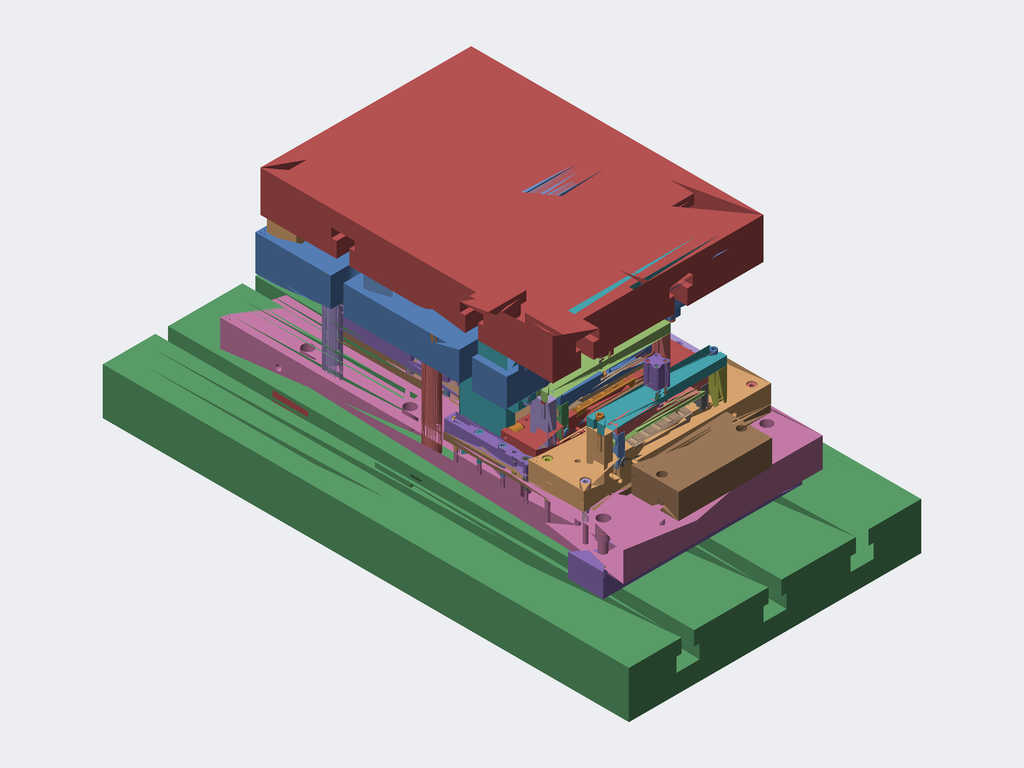Assembly | STEP file | 558 different items | 558 placed
Parts list (item | name | quantity | parent item | size | volume), first 318 of 558 items:
1 | 200 mesh_id1002 | x1 | in 200 mesh_xmt_txt | 10 x 10 x 26 mm | 909.194 mm3
2 | 200 mesh_id1006 | x1 | in 200 mesh_xmt_txt | 10 x 10 x 26 mm | 909.194 mm3
3 | 200 mesh_id1010 | x1 | in 200 mesh_xmt_txt | 10 x 10 x 26 mm | 909.194 mm3
4 | 200 mesh_id1014 | x1 | in 200 mesh_xmt_txt | 10 x 10 x 26 mm | 909.194 mm3
5 | 200 mesh_id1018 | x1 | in 200 mesh_xmt_txt | 10 x 10 x 26 mm | 909.194 mm3
6 | 200 mesh_id1022 | x1 | in 200 mesh_xmt_txt | 10 x 10 x 26 mm | 909.194 mm3
7 | 200 mesh_id1026 | x1 | in 200 mesh_xmt_txt | 10 x 10 x 21 mm | 806.082 mm3
8 | 200 mesh_id102_x | x1 | in 200 mesh_xmt_txt | 6 x 6 x 36.5 mm | 342.508 mm3
9 | 200 mesh_id1030 | x1 | in 200 mesh_xmt_txt | 10 x 10 x 21 mm | 806.082 mm3
10 | 200 mesh_id1034 | x1 | in 200 mesh_xmt_txt | 10 x 10 x 21 mm | 806.082 mm3
11 | 200 mesh_id1038 | x1 | in 200 mesh_xmt_txt | 10 x 10 x 21 mm | 806.082 mm3
12 | 200 mesh_id1042 | x1 | in 200 mesh_xmt_txt | 10 x 10 x 21 mm | 806.082 mm3
13 | 200 mesh_id1046 | x1 | in 200 mesh_xmt_txt | 6 x 6 x 24.2 mm | 255.883 mm3
14 | 200 mesh_id1050 | x1 | in 200 mesh_xmt_txt | 6 x 6 x 24.2 mm | 255.883 mm3
15 | 200 mesh_id1054 | x1 | in 200 mesh_xmt_txt | 6 x 6 x 24.2 mm | 255.883 mm3
16 | 200 mesh_id1058 | x1 | in 200 mesh_xmt_txt | 6 x 6 x 24.2 mm | 255.883 mm3
17 | 200 mesh_id1062 | x1 | in 200 mesh_xmt_txt | 6 x 6 x 24.2 mm | 255.883 mm3
18 | 200 mesh_id1066 | x1 | in 200 mesh_xmt_txt | 6 x 6 x 24.2 mm | 255.883 mm3
19 | 200 mesh_id106_x | x1 | in 200 mesh_xmt_txt | 6 x 6 x 36.5 mm | 342.508 mm3
20 | 200 mesh_id1070 | x1 | in 200 mesh_xmt_txt | 6 x 6 x 24.2 mm | 255.883 mm3
21 | 200 mesh_id1074 | x1 | in 200 mesh_xmt_txt | 6 x 6 x 24.2 mm | 255.883 mm3
22 | 200 mesh_id1078 | x1 | in 200 mesh_xmt_txt | 6 x 6 x 24.2 mm | 255.883 mm3
23 | 200 mesh_id1082 | x1 | in 200 mesh_xmt_txt | 6 x 6 x 24.2 mm | 255.883 mm3
24 | 200 mesh_id1086 | x1 | in 200 mesh_xmt_txt | 6 x 6 x 24.2 mm | 255.883 mm3
25 | 200 mesh_id1090 | x1 | in 200 mesh_xmt_txt | 6 x 6 x 24.2 mm | 255.883 mm3
26 | 200 mesh_id1094 | x1 | in 200 mesh_xmt_txt | 6 x 6 x 24.2 mm | 255.883 mm3
27 | 200 mesh_id1098 | x1 | in 200 mesh_xmt_txt | 6 x 6 x 24.2 mm | 255.883 mm3
28 | 200 mesh_id10_xmt | x1 | in 200 mesh_xmt_txt | 60 x 14 x 9.8 mm | 6516 mm3
29 | 200 mesh_id1102 | x1 | in 200 mesh_xmt_txt | 6 x 6 x 24.2 mm | 255.883 mm3
30 | 200 mesh_id1106 | x1 | in 200 mesh_xmt_txt | 6 x 6 x 24.2 mm | 255.883 mm3
31 | 200 mesh_id110_x | x1 | in 200 mesh_xmt_txt | 6 x 6 x 36.5 mm | 342.508 mm3
32 | 200 mesh_id1110 | x1 | in 200 mesh_xmt_txt | 6 x 6 x 24.2 mm | 255.883 mm3
33 | 200 mesh_id1114 | x1 | in 200 mesh_xmt_txt | 6 x 6 x 24.2 mm | 255.883 mm3
34 | 200 mesh_id1118 | x1 | in 200 mesh_xmt_txt | 6 x 6 x 33.5 mm | 321.621 mm3
35 | 200 mesh_id1122 | x1 | in 200 mesh_xmt_txt | 6 x 6 x 33.5 mm | 321.621 mm3
36 | 200 mesh_id1126 | x1 | in 200 mesh_xmt_txt | 6 x 6 x 33.5 mm | 321.621 mm3
37 | 200 mesh_id1130 | x1 | in 200 mesh_xmt_txt | 6 x 6 x 33.5 mm | 321.621 mm3
38 | 200 mesh_id1134 | x1 | in 200 mesh_xmt_txt | 6 x 6 x 33.5 mm | 321.621 mm3
39 | 200 mesh_id1138 | x1 | in 200 mesh_xmt_txt | 6 x 6 x 33.5 mm | 321.621 mm3
40 | 200 mesh_id1142 | x1 | in 200 mesh_xmt_txt | 6 x 6 x 33.5 mm | 321.621 mm3
41 | 200 mesh_id1146 | x1 | in 200 mesh_xmt_txt | 6 x 6 x 33.5 mm | 321.621 mm3
42 | 200 mesh_id114_x | x1 | in 200 mesh_xmt_txt | 6 x 6 x 36.5 mm | 342.508 mm3
43 | 200 mesh_id1150 | x1 | in 200 mesh_xmt_txt | 6 x 6 x 33.5 mm | 321.621 mm3
44 | 200 mesh_id1154 | x1 | in 200 mesh_xmt_txt | 6 x 6 x 33.5 mm | 321.621 mm3
45 | 200 mesh_id1158 | x1 | in 200 mesh_xmt_txt | 6 x 6 x 33.5 mm | 321.621 mm3
46 | 200 mesh_id1162 | x1 | in 200 mesh_xmt_txt | 6 x 6 x 33.5 mm | 321.621 mm3
47 | 200 mesh_id1166 | x1 | in 200 mesh_xmt_txt | 6 x 6 x 33.5 mm | 321.621 mm3
48 | 200 mesh_id1170 | x1 | in 200 mesh_xmt_txt | 6 x 6 x 33.5 mm | 321.621 mm3
49 | 200 mesh_id1174 | x1 | in 200 mesh_xmt_txt | 6 x 6 x 33.5 mm | 321.621 mm3
50 | 200 mesh_id1178 | x1 | in 200 mesh_xmt_txt | 6 x 6 x 33.5 mm | 321.621 mm3
51 | 200 mesh_id1182 | x1 | in 200 mesh_xmt_txt | 6 x 6 x 31.5 mm | 307.483 mm3
52 | 200 mesh_id1186 | x1 | in 200 mesh_xmt_txt | 6 x 6 x 31.5 mm | 307.483 mm3
53 | 200 mesh_id118_x | x1 | in 200 mesh_xmt_txt | 6 x 6 x 36.5 mm | 342.508 mm3
54 | 200 mesh_id1190 | x1 | in 200 mesh_xmt_txt | 6 x 6 x 31.5 mm | 307.483 mm3
55 | 200 mesh_id1194 | x1 | in 200 mesh_xmt_txt | 6 x 6 x 31.5 mm | 307.483 mm3
56 | 200 mesh_id1198 | x1 | in 200 mesh_xmt_txt | 6 x 6 x 31.5 mm | 307.483 mm3
57 | 200 mesh_id1202 | x1 | in 200 mesh_xmt_txt | 6 x 6 x 31.5 mm | 307.483 mm3
58 | 200 mesh_id1206 | x1 | in 200 mesh_xmt_txt | 6 x 6 x 31.5 mm | 307.483 mm3
59 | 200 mesh_id1210 | x1 | in 200 mesh_xmt_txt | 6 x 6 x 31.5 mm | 307.483 mm3
60 | 200 mesh_id1214 | x1 | in 200 mesh_xmt_txt | 6 x 6 x 31.5 mm | 307.483 mm3
61 | 200 mesh_id1218 | x1 | in 200 mesh_xmt_txt | 6 x 6 x 31.5 mm | 307.483 mm3
62 | 200 mesh_id1222 | x1 | in 200 mesh_xmt_txt | 6 x 6 x 31.5 mm | 307.483 mm3
63 | 200 mesh_id1226 | x1 | in 200 mesh_xmt_txt | 6 x 6 x 31.5 mm | 307.483 mm3
64 | 200 mesh_id122_x | x1 | in 200 mesh_xmt_txt | 8 x 8 x 55 mm | 2726 mm3
65 | 200 mesh_id1230 | x1 | in 200 mesh_xmt_txt | 6 x 6 x 31.5 mm | 307.483 mm3
66 | 200 mesh_id1234 | x1 | in 200 mesh_xmt_txt | 6 x 6 x 31.5 mm | 307.483 mm3
67 | 200 mesh_id1238 | x1 | in 200 mesh_xmt_txt | 10 x 10 x 21 mm | 805.584 mm3
68 | 200 mesh_id1242 | x1 | in 200 mesh_xmt_txt | 8.5 x 8.5 x 45 mm | 1026 mm3
69 | 200 mesh_id1246 | x1 | in 200 mesh_xmt_txt | 8.5 x 8.5 x 45 mm | 1026 mm3
70 | 200 mesh_id1250 | x1 | in 200 mesh_xmt_txt | 39.94 x 2.4 x 27.2 mm | 2495 mm3
71 | 200 mesh_id1254 | x1 | in 200 mesh_xmt_txt | 39.94 x 2.4 x 27.2 mm | 2495 mm3
72 | 200 mesh_id1258 | x1 | in 200 mesh_xmt_txt | 39.94 x 2.4 x 27.2 mm | 2495 mm3
73 | 200 mesh_id1262 | x1 | in 200 mesh_xmt_txt | 39.94 x 2.4 x 27.2 mm | 2495 mm3
74 | 200 mesh_id1266 | x1 | in 200 mesh_xmt_txt | 39.94 x 2.4 x 27.2 mm | 2495 mm3
75 | 200 mesh_id126_x | x1 | in 200 mesh_xmt_txt | 10 x 10 x 21 mm | 805.776 mm3
76 | 200 mesh_id1270 | x1 | in 200 mesh_xmt_txt | 39.94 x 2.4 x 27.2 mm | 2495 mm3
77 | 200 mesh_id1274 | x1 | in 200 mesh_xmt_txt | 39.94 x 2.4 x 27.2 mm | 2495 mm3
78 | 200 mesh_id1278 | x1 | in 200 mesh_xmt_txt | 39.94 x 2.4 x 27.2 mm | 2495 mm3
79 | 200 mesh_id1282 | x1 | in 200 mesh_xmt_txt | 39.94 x 2.4 x 27.2 mm | 2495 mm3
80 | 200 mesh_id1286 | x1 | in 200 mesh_xmt_txt | 39.94 x 2.4 x 27.2 mm | 2495 mm3
81 | 200 mesh_id1290 | x1 | in 200 mesh_xmt_txt | 39.94 x 2.4 x 27.2 mm | 2495 mm3
82 | 200 mesh_id1294 | x1 | in 200 mesh_xmt_txt | 39.94 x 2.4 x 27.2 mm | 2495 mm3
83 | 200 mesh_id1298 | x1 | in 200 mesh_xmt_txt | 39.94 x 2.4 x 27.2 mm | 2495 mm3
84 | 200 mesh_id1302 | x1 | in 200 mesh_xmt_txt | 39.94 x 2.4 x 27.2 mm | 2495 mm3
85 | 200 mesh_id1306 | x1 | in 200 mesh_xmt_txt | 39.94 x 2.4 x 27.2 mm | 2495 mm3
86 | 200 mesh_id130_x | x1 | in 200 mesh_xmt_txt | 8.5 x 8.5 x 20 mm | 535.142 mm3
87 | 200 mesh_id1310 | x1 | in 200 mesh_xmt_txt | 39.94 x 2.4 x 27.2 mm | 2495 mm3
88 | 200 mesh_id1314 | x1 | in 200 mesh_xmt_txt | 39.94 x 2.4 x 27.2 mm | 2495 mm3
89 | 200 mesh_id1318 | x1 | in 200 mesh_xmt_txt | 39.94 x 2.4 x 27.2 mm | 2495 mm3
90 | 200 mesh_id1322 | x1 | in 200 mesh_xmt_txt | 22 x 22 x 5 mm | 1608 mm3
91 | 200 mesh_id1326 | x1 | in 200 mesh_xmt_txt | 12 x 12 x 32.3 mm | 2576 mm3
92 | 200 mesh_id1330 | x1 | in 200 mesh_xmt_txt | 12 x 12 x 32.3 mm | 2576 mm3
93 | 200 mesh_id1334 | x1 | in 200 mesh_xmt_txt | 22 x 22 x 5 mm | 1608 mm3
94 | 200 mesh_id1338 | x1 | in 200 mesh_xmt_txt | 12 x 12 x 32.3 mm | 2576 mm3
95 | 200 mesh_id1342 | x1 | in 200 mesh_xmt_txt | 22 x 22 x 5 mm | 1608 mm3
96 | 200 mesh_id1346 | x1 | in 200 mesh_xmt_txt | 12 x 12 x 32.3 mm | 2576 mm3
97 | 200 mesh_id134_x | x1 | in 200 mesh_xmt_txt | 10 x 10 x 51 mm | 1654 mm3
98 | 200 mesh_id1350 | x1 | in 200 mesh_xmt_txt | 22 x 22 x 5 mm | 1608 mm3
99 | 200 mesh_id1354 | x1 | in 200 mesh_xmt_txt | 22 x 22 x 5 mm | 1608 mm3
100 | 200 mesh_id1358 | x1 | in 200 mesh_xmt_txt | 12 x 12 x 32.3 mm | 2576 mm3
101 | 200 mesh_id1362 | x1 | in 200 mesh_xmt_txt | 22 x 22 x 5 mm | 1608 mm3
102 | 200 mesh_id1366 | x1 | in 200 mesh_xmt_txt | 12 x 12 x 32.3 mm | 2576 mm3
103 | 200 mesh_id1370 | x1 | in 200 mesh_xmt_txt | 8 x 8 x 10 mm | 413.018 mm3
104 | 200 mesh_id1374 | x1 | in 200 mesh_xmt_txt | 8 x 8 x 10 mm | 413.018 mm3
105 | 200 mesh_id1378 | x1 | in 200 mesh_xmt_txt | 8 x 8 x 10 mm | 413.018 mm3
106 | 200 mesh_id1382 | x1 | in 200 mesh_xmt_txt | 8 x 8 x 10 mm | 413.018 mm3
107 | 200 mesh_id1386 | x1 | in 200 mesh_xmt_txt | 8 x 8 x 10 mm | 413.018 mm3
108 | 200 mesh_id138_x | x1 | in 200 mesh_xmt_txt | 18 x 18 x 30 mm | 2880 mm3
109 | 200 mesh_id1390 | x1 | in 200 mesh_xmt_txt | 8 x 8 x 10 mm | 413.018 mm3
110 | 200 mesh_id1394 | x1 | in 200 mesh_xmt_txt | 8 x 8 x 10 mm | 413.018 mm3
111 | 200 mesh_id1398 | x1 | in 200 mesh_xmt_txt | 8 x 8 x 10 mm | 413.018 mm3
112 | 200 mesh_id1402 | x1 | in 200 mesh_xmt_txt | 8 x 8 x 10 mm | 413.018 mm3
113 | 200 mesh_id1406 | x1 | in 200 mesh_xmt_txt | 8 x 8 x 10 mm | 413.018 mm3
114 | 200 mesh_id1410 | x1 | in 200 mesh_xmt_txt | 8 x 8 x 10 mm | 413.018 mm3
115 | 200 mesh_id1414 | x1 | in 200 mesh_xmt_txt | 8 x 8 x 10 mm | 413.018 mm3
116 | 200 mesh_id1418 | x1 | in 200 mesh_xmt_txt | 8 x 8 x 10 mm | 413.018 mm3
117 | 200 mesh_id1422 | x1 | in 200 mesh_xmt_txt | 8 x 8 x 10 mm | 413.018 mm3
118 | 200 mesh_id1426 | x1 | in 200 mesh_xmt_txt | 8 x 8 x 10 mm | 413.018 mm3
119 | 200 mesh_id142_x | x1 | in 200 mesh_xmt_txt | 18 x 18 x 30 mm | 2880 mm3
120 | 200 mesh_id1430 | x1 | in 200 mesh_xmt_txt | 8 x 8 x 10 mm | 413.018 mm3
121 | 200 mesh_id1434 | x1 | in 200 mesh_xmt_txt | 8 x 8 x 10 mm | 413.018 mm3
122 | 200 mesh_id1438 | x1 | in 200 mesh_xmt_txt | 8 x 8 x 10 mm | 413.018 mm3
123 | 200 mesh_id1442 | x1 | in 200 mesh_xmt_txt | 8 x 8 x 10 mm | 413.018 mm3
124 | 200 mesh_id1446 | x1 | in 200 mesh_xmt_txt | 8 x 8 x 10 mm | 413.018 mm3
125 | 200 mesh_id1450 | x1 | in 200 mesh_xmt_txt | 8 x 8 x 10 mm | 413.018 mm3
126 | 200 mesh_id1454 | x1 | in 200 mesh_xmt_txt | 8 x 8 x 10 mm | 413.018 mm3
127 | 200 mesh_id1458 | x1 | in 200 mesh_xmt_txt | 8 x 8 x 10 mm | 413.018 mm3
128 | 200 mesh_id1462 | x1 | in 200 mesh_xmt_txt | 8 x 8 x 10 mm | 413.018 mm3
129 | 200 mesh_id1466 | x1 | in 200 mesh_xmt_txt | 8 x 8 x 10 mm | 413.018 mm3
130 | 200 mesh_id146_x | x1 | in 200 mesh_xmt_txt | 18 x 18 x 30 mm | 2880 mm3
131 | 200 mesh_id1470 | x1 | in 200 mesh_xmt_txt | 8 x 8 x 10 mm | 413.018 mm3
132 | 200 mesh_id1474 | x1 | in 200 mesh_xmt_txt | 8 x 8 x 10 mm | 413.018 mm3
133 | 200 mesh_id1478 | x1 | in 200 mesh_xmt_txt | 8 x 8 x 10 mm | 413.018 mm3
134 | 200 mesh_id1482 | x1 | in 200 mesh_xmt_txt | 8 x 8 x 10 mm | 413.018 mm3
135 | 200 mesh_id1486 | x1 | in 200 mesh_xmt_txt | 8 x 8 x 10 mm | 413.018 mm3
136 | 200 mesh_id1490 | x1 | in 200 mesh_xmt_txt | 8 x 8 x 10 mm | 413.018 mm3
137 | 200 mesh_id1494 | x1 | in 200 mesh_xmt_txt | 8 x 8 x 10 mm | 413.018 mm3
138 | 200 mesh_id1498 | x1 | in 200 mesh_xmt_txt | 8 x 8 x 10 mm | 413.018 mm3
139 | 200 mesh_id14_xmt | x1 | in 200 mesh_xmt_txt | 34.97 x 6 x 32.7 mm | 4654 mm3
140 | 200 mesh_id1502 | x1 | in 200 mesh_xmt_txt | 8 x 8 x 10 mm | 413.018 mm3
141 | 200 mesh_id1506 | x1 | in 200 mesh_xmt_txt | 8 x 8 x 10 mm | 413.018 mm3
142 | 200 mesh_id150_x | x1 | in 200 mesh_xmt_txt | 18 x 18 x 30 mm | 2880 mm3
143 | 200 mesh_id1510 | x1 | in 200 mesh_xmt_txt | 8 x 8 x 10 mm | 413.018 mm3
144 | 200 mesh_id1514 | x1 | in 200 mesh_xmt_txt | 8 x 8 x 10 mm | 413.018 mm3
145 | 200 mesh_id1518 | x1 | in 200 mesh_xmt_txt | 8 x 8 x 10 mm | 413.018 mm3
146 | 200 mesh_id1522 | x1 | in 200 mesh_xmt_txt | 8 x 8 x 10 mm | 413.018 mm3
147 | 200 mesh_id1526 | x1 | in 200 mesh_xmt_txt | 8 x 8 x 10 mm | 413.018 mm3
148 | 200 mesh_id1530 | x1 | in 200 mesh_xmt_txt | 8 x 8 x 10 mm | 413.018 mm3
149 | 200 mesh_id1534 | x1 | in 200 mesh_xmt_txt | 8 x 8 x 10 mm | 413.018 mm3
150 | 200 mesh_id1538 | x1 | in 200 mesh_xmt_txt | 8 x 8 x 10 mm | 413.018 mm3
151 | 200 mesh_id1542 | x1 | in 200 mesh_xmt_txt | 8 x 8 x 10 mm | 413.018 mm3
152 | 200 mesh_id1546 | x1 | in 200 mesh_xmt_txt | 8 x 8 x 10 mm | 413.018 mm3
153 | 200 mesh_id154_x | x1 | in 200 mesh_xmt_txt | 18 x 18 x 30 mm | 2880 mm3
154 | 200 mesh_id1550 | x1 | in 200 mesh_xmt_txt | 8 x 8 x 10 mm | 413.018 mm3
155 | 200 mesh_id1554 | x1 | in 200 mesh_xmt_txt | 8 x 8 x 10 mm | 413.018 mm3
156 | 200 mesh_id1558 | x1 | in 200 mesh_xmt_txt | 24.97 x 5.97 x 53 mm | 7855 mm3
157 | 200 mesh_id1562 | x1 | in 200 mesh_xmt_txt | 6 x 6 x 40 mm | 281.63 mm3
158 | 200 mesh_id1566 | x1 | in 200 mesh_xmt_txt | 6 x 6 x 40 mm | 281.63 mm3
159 | 200 mesh_id1570 | x1 | in 200 mesh_xmt_txt | 6 x 6 x 40 mm | 281.63 mm3
160 | 200 mesh_id1574 | x1 | in 200 mesh_xmt_txt | 6 x 6 x 40 mm | 281.63 mm3
161 | 200 mesh_id1578 | x1 | in 200 mesh_xmt_txt | 6 x 6 x 40 mm | 281.63 mm3
162 | 200 mesh_id1582 | x1 | in 200 mesh_xmt_txt | 6 x 6 x 40 mm | 281.63 mm3
163 | 200 mesh_id1586 | x1 | in 200 mesh_xmt_txt | 6 x 6 x 40 mm | 281.63 mm3
164 | 200 mesh_id158_x | x1 | in 200 mesh_xmt_txt | 18 x 18 x 30 mm | 2880 mm3
165 | 200 mesh_id1590 | x1 | in 200 mesh_xmt_txt | 6 x 6 x 40 mm | 281.63 mm3
166 | 200 mesh_id1594 | x1 | in 200 mesh_xmt_txt | 6 x 6 x 40 mm | 281.63 mm3
167 | 200 mesh_id1598 | x1 | in 200 mesh_xmt_txt | 6 x 6 x 40 mm | 281.63 mm3
168 | 200 mesh_id1602 | x1 | in 200 mesh_xmt_txt | 6 x 6 x 40 mm | 281.63 mm3
169 | 200 mesh_id1606 | x1 | in 200 mesh_xmt_txt | 6 x 6 x 40 mm | 281.63 mm3
170 | 200 mesh_id1610 | x1 | in 200 mesh_xmt_txt | 6 x 6 x 40 mm | 281.63 mm3
171 | 200 mesh_id1614 | x1 | in 200 mesh_xmt_txt | 6 x 6 x 40 mm | 281.63 mm3
172 | 200 mesh_id1618 | x1 | in 200 mesh_xmt_txt | - | 70.891 mm3
173 | 200 mesh_id1622 | x1 | in 200 mesh_xmt_txt | - | 70.891 mm3
174 | 200 mesh_id1626 | x1 | in 200 mesh_xmt_txt | - | 70.891 mm3
175 | 200 mesh_id162_x | x1 | in 200 mesh_xmt_txt | 25 x 25 x 5 mm | 2168 mm3
176 | 200 mesh_id1630 | x1 | in 200 mesh_xmt_txt | - | 70.891 mm3
177 | 200 mesh_id1634 | x1 | in 200 mesh_xmt_txt | - | 70.891 mm3
178 | 200 mesh_id1638 | x1 | in 200 mesh_xmt_txt | - | 70.891 mm3
179 | 200 mesh_id1642 | x1 | in 200 mesh_xmt_txt | - | 70.891 mm3
180 | 200 mesh_id1646 | x1 | in 200 mesh_xmt_txt | - | 70.891 mm3
181 | 200 mesh_id1650 | x1 | in 200 mesh_xmt_txt | - | 70.891 mm3
182 | 200 mesh_id1654 | x1 | in 200 mesh_xmt_txt | - | 70.891 mm3
183 | 200 mesh_id1658 | x1 | in 200 mesh_xmt_txt | - | 70.891 mm3
184 | 200 mesh_id1662 | x1 | in 200 mesh_xmt_txt | - | 70.891 mm3
185 | 200 mesh_id1666 | x1 | in 200 mesh_xmt_txt | - | 70.891 mm3
186 | 200 mesh_id166_x | x1 | in 200 mesh_xmt_txt | 16 x 16 x 25 mm | 3601 mm3
187 | 200 mesh_id1670 | x1 | in 200 mesh_xmt_txt | - | 70.891 mm3
188 | 200 mesh_id1674 | x1 | in 200 mesh_xmt_txt | - | 70.891 mm3
189 | 200 mesh_id1678 | x1 | in 200 mesh_xmt_txt | - | 70.891 mm3
190 | 200 mesh_id1682 | x1 | in 200 mesh_xmt_txt | - | 70.891 mm3
191 | 200 mesh_id1686 | x1 | in 200 mesh_xmt_txt | - | 65.446 mm3
192 | 200 mesh_id1690 | x1 | in 200 mesh_xmt_txt | - | 65.446 mm3
193 | 200 mesh_id1694 | x1 | in 200 mesh_xmt_txt | - | 65.446 mm3
194 | 200 mesh_id1698 | x1 | in 200 mesh_xmt_txt | - | 65.446 mm3
195 | 200 mesh_id1702 | x1 | in 200 mesh_xmt_txt | - | 65.446 mm3
196 | 200 mesh_id1706 | x1 | in 200 mesh_xmt_txt | - | 65.446 mm3
197 | 200 mesh_id170_x | x1 | in 200 mesh_xmt_txt | 25 x 25 x 5 mm | 2168 mm3
198 | 200 mesh_id1710 | x1 | in 200 mesh_xmt_txt | - | 65.446 mm3
199 | 200 mesh_id1714 | x1 | in 200 mesh_xmt_txt | - | 65.446 mm3
200 | 200 mesh_id1718 | x1 | in 200 mesh_xmt_txt | - | 65.446 mm3
201 | 200 mesh_id1722 | x1 | in 200 mesh_xmt_txt | - | 65.446 mm3
202 | 200 mesh_id1726 | x1 | in 200 mesh_xmt_txt | - | 65.446 mm3
203 | 200 mesh_id1730 | x1 | in 200 mesh_xmt_txt | - | 65.446 mm3
204 | 200 mesh_id1734 | x1 | in 200 mesh_xmt_txt | - | 65.446 mm3
205 | 200 mesh_id1738 | x1 | in 200 mesh_xmt_txt | - | 65.446 mm3
206 | 200 mesh_id1742 | x1 | in 200 mesh_xmt_txt | - | 65.446 mm3
207 | 200 mesh_id1746 | x1 | in 200 mesh_xmt_txt | - | 65.446 mm3
208 | 200 mesh_id174_x | x1 | in 200 mesh_xmt_txt | 16 x 16 x 25 mm | 3601 mm3
209 | 200 mesh_id1750 | x1 | in 200 mesh_xmt_txt | - | 65.446 mm3
210 | 200 mesh_id1754 | x1 | in 200 mesh_xmt_txt | - | 65.446 mm3
211 | 200 mesh_id1758 | x1 | in 200 mesh_xmt_txt | 25 x 25 x 45 mm | 5947 mm3
212 | 200 mesh_id1762 | x1 | in 200 mesh_xmt_txt | 25 x 25 x 45 mm | 5947 mm3
213 | 200 mesh_id1766 | x1 | in 200 mesh_xmt_txt | 25 x 25 x 45 mm | 5947 mm3
214 | 200 mesh_id1770 | x1 | in 200 mesh_xmt_txt | 25 x 25 x 45 mm | 5947 mm3
215 | 200 mesh_id1774 | x1 | in 200 mesh_xmt_txt | 25 x 25 x 45 mm | 5947 mm3
216 | 200 mesh_id1778 | x1 | in 200 mesh_xmt_txt | 25 x 25 x 45 mm | 5947 mm3
217 | 200 mesh_id1782 | x1 | in 200 mesh_xmt_txt | 25 x 25 x 45 mm | 5947 mm3
218 | 200 mesh_id1786 | x1 | in 200 mesh_xmt_txt | 25 x 25 x 45 mm | 5947 mm3
219 | 200 mesh_id178_x | x1 | in 200 mesh_xmt_txt | 25 x 25 x 5 mm | 2168 mm3
220 | 200 mesh_id1790 | x1 | in 200 mesh_xmt_txt | 28 x 28 x 30 mm | 6929 mm3
221 | 200 mesh_id1794 | x1 | in 200 mesh_xmt_txt | 22 x 21.896 x 30 mm | 3861 mm3
222 | 200 mesh_id1798 | x1 | in 200 mesh_xmt_txt | 23 x 23 x 140 mm | 28914 mm3
223 | 200 mesh_id1802 | x1 | in 200 mesh_xmt_txt | 21.896 x 22 x 30 mm | 3781 mm3
224 | 200 mesh_id1806 | x1 | in 200 mesh_xmt_txt | 28 x 28 x 35 mm | 8107 mm3
225 | 200 mesh_id1810 | x1 | in 200 mesh_xmt_txt | 28 x 28 x 35 mm | 8107 mm3
226 | 200 mesh_id1814 | x1 | in 200 mesh_xmt_txt | 23 x 23 x 140 mm | 28914 mm3
227 | 200 mesh_id1818 | x1 | in 200 mesh_xmt_txt | 21.896 x 22 x 30 mm | 3781 mm3
228 | 200 mesh_id1822 | x1 | in 200 mesh_xmt_txt | 28 x 28 x 30 mm | 6929 mm3
229 | 200 mesh_id1826 | x1 | in 200 mesh_xmt_txt | 22 x 21.896 x 30 mm | 3861 mm3
230 | 200 mesh_id182_x | x1 | in 200 mesh_xmt_txt | 16 x 16 x 25 mm | 3601 mm3
231 | 200 mesh_id1830 | x1 | in 200 mesh_xmt_txt | 28 x 28 x 35 mm | 8107 mm3
232 | 200 mesh_id1834 | x1 | in 200 mesh_xmt_txt | 23 x 23 x 140 mm | 28914 mm3
233 | 200 mesh_id1838 | x1 | in 200 mesh_xmt_txt | 21.896 x 22 x 30 mm | 3781 mm3
234 | 200 mesh_id1842 | x1 | in 200 mesh_xmt_txt | 22 x 21.896 x 30 mm | 3861 mm3
235 | 200 mesh_id1846 | x1 | in 200 mesh_xmt_txt | 28 x 28 x 30 mm | 6929 mm3
236 | 200 mesh_id1850 | x1 | in 200 mesh_xmt_txt | 28 x 28 x 30 mm | 6929 mm3
237 | 200 mesh_id1854 | x1 | in 200 mesh_xmt_txt | 22 x 21.896 x 30 mm | 3861 mm3
238 | 200 mesh_id1858 | x1 | in 200 mesh_xmt_txt | 23 x 23 x 140 mm | 28914 mm3
239 | 200 mesh_id1862 | x1 | in 200 mesh_xmt_txt | 28 x 28 x 35 mm | 8107 mm3
240 | 200 mesh_id1866 | x1 | in 200 mesh_xmt_txt | 21.896 x 22 x 30 mm | 3781 mm3
241 | 200 mesh_id186_x | x1 | in 200 mesh_xmt_txt | 25 x 25 x 5 mm | 2168 mm3
242 | 200 mesh_id1870 | x1 | in 200 mesh_xmt_txt | 75.6 x 4.94 x 20.309 mm | 3191 mm3
243 | 200 mesh_id1874 | x1 | in 200 mesh_xmt_txt | 75.6 x 4.94 x 20.309 mm | 3191 mm3
244 | 200 mesh_id1878 | x1 | in 200 mesh_xmt_txt | 75.6 x 4.94 x 20.309 mm | 3191 mm3
245 | 200 mesh_id1882 | x1 | in 200 mesh_xmt_txt | 75.6 x 4.94 x 20.309 mm | 3191 mm3
246 | 200 mesh_id1886 | x1 | in 200 mesh_xmt_txt | 90 x 4.94 x 26.94 mm | 4137 mm3
247 | 200 mesh_id1890 | x1 | in 200 mesh_xmt_txt | 90 x 4.94 x 26.94 mm | 4137 mm3
248 | 200 mesh_id1894 | x1 | in 200 mesh_xmt_txt | 90 x 4.94 x 26.94 mm | 4137 mm3
249 | 200 mesh_id1898 | x1 | in 200 mesh_xmt_txt | 90 x 4.94 x 26.94 mm | 4137 mm3
250 | 200 mesh_id18_xmt | x1 | in 200 mesh_xmt_txt | 34.97 x 6 x 32.7 mm | 4654 mm3
251 | 200 mesh_id1902 | x1 | in 200 mesh_xmt_txt | 109.8 x 2.8 x 28.9 mm | 4981 mm3
252 | 200 mesh_id1906 | x1 | in 200 mesh_xmt_txt | 109.8 x 2.8 x 28.9 mm | 4981 mm3
253 | 200 mesh_id190_x | x1 | in 200 mesh_xmt_txt | 16 x 16 x 25 mm | 3601 mm3
254 | 200 mesh_id1910 | x1 | in 200 mesh_xmt_txt | 109.8 x 2.8 x 28.9 mm | 4981 mm3
255 | 200 mesh_id1914 | x1 | in 200 mesh_xmt_txt | 20 x 156 x 20 mm | 54101 mm3
256 | 200 mesh_id1918 | x1 | in 200 mesh_xmt_txt | 22 x 100 x 30.627 mm | 61945 mm3
257 | 200 mesh_id1922 | x1 | in 200 mesh_xmt_txt | 140 x 20 x 20 mm | 44533 mm3
258 | 200 mesh_id1926 | x1 | in 200 mesh_xmt_txt | 20 x 156 x 20 mm | 54101 mm3
259 | 200 mesh_id1930 | x1 | in 200 mesh_xmt_txt | 14 x 155 x 7.945 mm | 13826 mm3
260 | 200 mesh_id1934 | x1 | in 200 mesh_xmt_txt | 22 x 17 x 50.8 mm | 12732 mm3
261 | 200 mesh_id1938 | x1 | in 200 mesh_xmt_txt | 30 x 15 x 75 mm | 33075 mm3
262 | 200 mesh_id1942 | x1 | in 200 mesh_xmt_txt | 30 x 210 x 15 mm | 89577 mm3
263 | 200 mesh_id1946 | x1 | in 200 mesh_xmt_txt | 30 x 15 x 75 mm | 33075 mm3
264 | 200 mesh_id194_x | x1 | in 200 mesh_xmt_txt | 25 x 25 x 5 mm | 2168 mm3
265 | 200 mesh_id1950 | x1 | in 200 mesh_xmt_txt | 22 x 17 x 50.8 mm | 12732 mm3
266 | 200 mesh_id1954 | x1 | in 200 mesh_xmt_txt | 18 x 18 x 9.92 mm | 1371 mm3
267 | 200 mesh_id1958 | x1 | in 200 mesh_xmt_txt | 12 x 12 x 46 mm | 1731 mm3
268 | 200 mesh_id1962 | x1 | in 200 mesh_xmt_txt | 25 x 25 x 37 mm | 14578 mm3
269 | 200 mesh_id1966 | x1 | in 200 mesh_xmt_txt | 25 x 25 x 37 mm | 14578 mm3
270 | 200 mesh_id1970 | x1 | in 200 mesh_xmt_txt | 12 x 12 x 46 mm | 1731 mm3
271 | 200 mesh_id1974 | x1 | in 200 mesh_xmt_txt | 18 x 18 x 9.92 mm | 1371 mm3
272 | 200 mesh_id1978 | x1 | in 200 mesh_xmt_txt | 150 x 150 x 43 mm | 782567 mm3
273 | 200 mesh_id1982 | x1 | in 200 mesh_xmt_txt | 25 x 16 x 80 mm | 27373 mm3
274 | 200 mesh_id1986 | x1 | in 200 mesh_xmt_txt | 25 x 16 x 80 mm | 27373 mm3
275 | 200 mesh_id198_x | x1 | in 200 mesh_xmt_txt | 16 x 16 x 25 mm | 3601 mm3
276 | 200 mesh_id1990 | x1 | in 200 mesh_xmt_txt | 25 x 105.8 x 15 mm | 37116 mm3
277 | 200 mesh_id1994 | x1 | in 200 mesh_xmt_txt | 25 x 130 x 15 mm | 46833 mm3
278 | 200 mesh_id1998 | x1 | in 200 mesh_xmt_txt | 50 x 360 x 20 mm | 353388 mm3
279 | 200 mesh_id2002 | x1 | in 200 mesh_xmt_txt | 50 x 360 x 20 mm | 331105 mm3
280 | 200 mesh_id2006 | x1 | in 200 mesh_xmt_txt | 50 x 360 x 20 mm | 353388 mm3
281 | 200 mesh_id2010 | x1 | in 200 mesh_xmt_txt | 75.6 x 4.94 x 20.309 mm | 3191 mm3
282 | 200 mesh_id2014 | x1 | in 200 mesh_xmt_txt | 115.071 x 4.98 x 53.4 mm | 17394 mm3
283 | 200 mesh_id2018 | x1 | in 200 mesh_xmt_txt | 115.071 x 4.98 x 53.4 mm | 17394 mm3
284 | 200 mesh_id2022 | x1 | in 200 mesh_xmt_txt | 250 x 210 x 20 mm | 913405 mm3
285 | 200 mesh_id2026 | x1 | in 200 mesh_xmt_txt | 250 x 210 x 25 mm | 669439 mm3
286 | 200 mesh_id202_x | x1 | in 200 mesh_xmt_txt | 25 x 25 x 5 mm | 2168 mm3
287 | 200 mesh_id2030 | x1 | in 200 mesh_xmt_txt | 500 x 360 x 70 mm | 11688110 mm3
288 | 200 mesh_id2034 | x1 | in 200 mesh_xmt_txt | 900 x 500 x 80 mm | 31982400 mm3
289 | 200 mesh_id2038 | x1 | in 200 mesh_xmt_txt | 109.8 x 2.8 x 28.9 mm | 4981 mm3
290 | 200 mesh_id2042 | x1 | in 200 mesh_xmt_txt | 131 x 16 x 210 mm | 283448 mm3
291 | 200 mesh_id2046 | x1 | in 200 mesh_xmt_txt | 115.071 x 4.98 x 53.4 mm | 17362 mm3
292 | 200 mesh_id2050 | x1 | in 200 mesh_xmt_txt | 115.071 x 4.98 x 53.4 mm | 17357 mm3
293 | 200 mesh_id2054 | x1 | in 200 mesh_xmt_txt | 78.34 x 4.98 x 24.75 mm | 4951 mm3
294 | 200 mesh_id2058 | x1 | in 200 mesh_xmt_txt | 78.34 x 4.98 x 24.75 mm | 4951 mm3
295 | 200 mesh_id2062 | x1 | in 200 mesh_xmt_txt | 78.34 x 4.98 x 24.75 mm | 4951 mm3
296 | 200 mesh_id2066 | x1 | in 200 mesh_xmt_txt | 78.34 x 4.98 x 24.75 mm | 4951 mm3
297 | 200 mesh_id206_x | x1 | in 200 mesh_xmt_txt | 16 x 16 x 25 mm | 3601 mm3
298 | 200 mesh_id2070 | x1 | in 200 mesh_xmt_txt | 135 x 135 x 15.259 mm | 197711 mm3
299 | 200 mesh_id2074 | x1 | in 200 mesh_xmt_txt | 135 x 121 x 21.89 mm | 302642 mm3
300 | 200 mesh_id2078 | x1 | in 200 mesh_xmt_txt | 115.071 x 4.98 x 53.4 mm | 17394 mm3
301 | 200 mesh_id2082 | x1 | in 200 mesh_xmt_txt | 690 x 340 x 50 mm | 10962643 mm3
302 | 200 mesh_id2086 | x1 | in 200 mesh_xmt_txt | 240 x 320 x 12 mm | 859349 mm3
303 | 200 mesh_id2090 | x1 | in 200 mesh_xmt_txt | 250 x 210 x 20 mm | 615513 mm3
304 | 200 mesh_id2094 | x1 | in 200 mesh_xmt_txt | 250 x 210 x 12 mm | 486087 mm3
305 | 200 mesh_id2098 | x1 | in 200 mesh_xmt_txt | 250 x 210 x 20 mm | 863809 mm3
306 | 200 mesh_id2102 | x1 | in 200 mesh_xmt_txt | 250 x 210 x 14 mm | 588514 mm3
307 | 200 mesh_id2106 | x1 | in 200 mesh_xmt_txt | 430 x 380 x 50 mm | 6493004 mm3
308 | 200 mesh_id210_x | x1 | in 200 mesh_xmt_txt | 25 x 25 x 5 mm | 2168 mm3
309 | 200 mesh_id2110 | x1 | in 200 mesh_xmt_txt | 135.01 x 135.01 x 10 mm | 121215 mm3
310 | 200 mesh_id2114 | x1 | in 200 mesh_xmt_txt | 24 x 20 x 22.9 mm | 7784 mm3
311 | 200 mesh_id2118 | x1 | in 200 mesh_xmt_txt | 24 x 20 x 22.9 mm | 7784 mm3
312 | 200 mesh_id2122 | x1 | in 200 mesh_xmt_txt | 117 x 1.9 x 19 mm | 2704 mm3
313 | 200 mesh_id2126 | x1 | in 200 mesh_xmt_txt | 117 x 1.9 x 19 mm | 2704 mm3
314 | 200 mesh_id2130 | x1 | in 200 mesh_xmt_txt | 117 x 1.9 x 19 mm | 2704 mm3
315 | 200 mesh_id2134 | x1 | in 200 mesh_xmt_txt | 117 x 1.9 x 19 mm | 2704 mm3
316 | 200 mesh_id2138 | x1 | in 200 mesh_xmt_txt | 117 x 1.9 x 19 mm | 2704 mm3
317 | 200 mesh_id2142 | x1 | in 200 mesh_xmt_txt | 117 x 1.9 x 19 mm | 2704 mm3
318 | 200 mesh_id2146 | x1 | in 200 mesh_xmt_txt | 117 x 1.9 x 19 mm | 2704 mm3